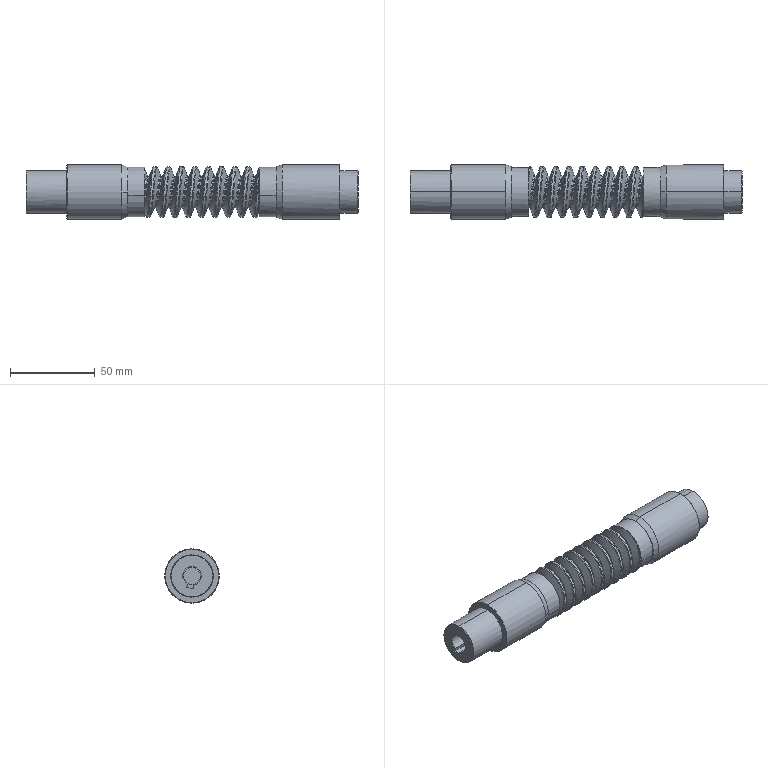Part | STEP file | 2026.6.15-Main Assembly图.sldasm-Part-133 | 1 solid | 91 faces | box 195.75 x 32 x 32 mm | volume 119299 mm3 | cylinder 54 | cone 16 | plane 15 | spline 6 | commonest cylinder face diameters 18.753 x19 30.003 x19 25 x4 29 x4 32 x4 10 x2